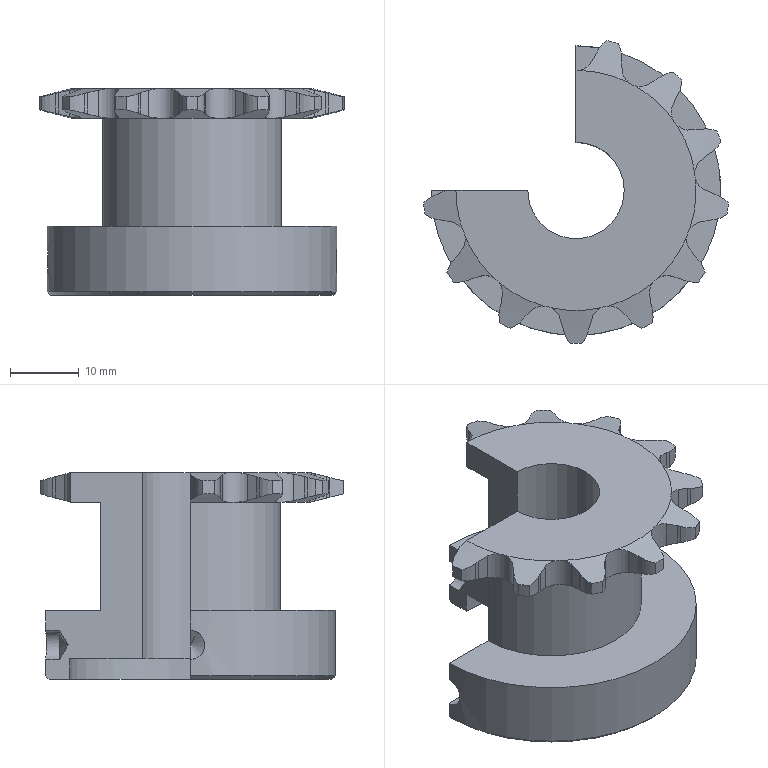Part | STEP file | driven sprocket | 1 solid | 132 faces | box 44.21 x 43.904 x 30.003 mm | volume 14979 mm3 | cylinder 78 | cone 27 | plane 27 | commonest cylinder face diameters 8.57 x21 13.236 x21 5.108 x14 44.359 x10 4.2 x4 14 x2